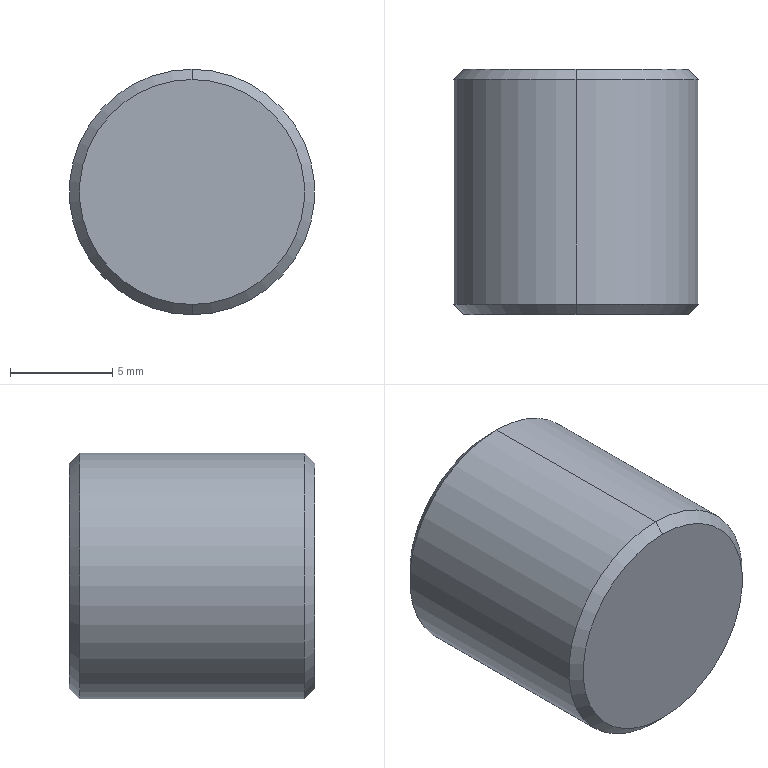Part | NX | features solid 2 | 1 solid | 20 faces | box 12 x 12 x 12 mm | volume 1208 mm3 | plane 14 | cone 4 | cylinder 2 | commonest cylinder face diameters 12 x2
STEP:
#1=CARTESIAN_POINT('',(240.5,-206.,53.));
#2=VERTEX_POINT('',#1);
#3=CARTESIAN_POINT('',(240.5,-206.,42.));
#4=VERTEX_POINT('',#3);
#5=CARTESIAN_POINT('',(240.5,-206.,47.5));
#6=DIRECTION('',(0.,1.,0.));
#7=DIRECTION('',(0.,0.,1.));
#8=AXIS2_PLACEMENT_3D('',#5,#6,#7);
#9=CIRCLE('',#8,5.5);
#10=EDGE_CURVE('',#2,#4,#9,.T.);
#11=ORIENTED_EDGE('',*,*,#10,.F.);
#12=CARTESIAN_POINT('',(240.5,-206.,47.5));
#13=DIRECTION('',(0.,-1.,0.));
#14=DIRECTION('',(0.,0.,1.));
#15=AXIS2_PLACEMENT_3D('',#12,#13,#14);
#16=CIRCLE('',#15,5.5);
#17=EDGE_CURVE('',#2,#4,#16,.T.);
#18=ORIENTED_EDGE('',*,*,#17,.T.);
#19=EDGE_LOOP('',(#11,#18));
#20=FACE_BOUND('',#19,.T.);
#21=CARTESIAN_POINT('',(240.5,-206.,47.5));
#22=DIRECTION('',(0.,1.,0.));
#23=DIRECTION('',(0.,0.,-1.));
#24=AXIS2_PLACEMENT_3D('',#21,#22,#23);
#25=PLANE('',#24);
#26=ADVANCED_FACE('',(#20),#25,.F.);
#27=CARTESIAN_POINT('',(240.5,-205.5,53.5));
#28=VERTEX_POINT('',#27);
#29=CARTESIAN_POINT('',(240.5,-206.,53.));
#30=DIRECTION('',(0.,0.7071,0.7071));
#31=VECTOR('',#30,1000.);
#32=LINE('',#29,#31);
#33=EDGE_CURVE('',#28,#2,#32,.F.);
#34=ORIENTED_EDGE('',*,*,#33,.F.);
#35=CARTESIAN_POINT('',(240.5,-205.5,41.5));
#36=VERTEX_POINT('',#35);
#37=CARTESIAN_POINT('',(240.5,-205.5,47.5));
#38=DIRECTION('',(0.,-1.,0.));
#39=DIRECTION('',(0.,0.,1.));
#40=AXIS2_PLACEMENT_3D('',#37,#38,#39);
#41=CIRCLE('',#40,6.);
#42=EDGE_CURVE('',#28,#36,#41,.T.);
#43=ORIENTED_EDGE('',*,*,#42,.T.);
#44=CARTESIAN_POINT('',(240.5,-206.,42.));
#45=DIRECTION('',(0.,0.7071,-0.7071));
#46=VECTOR('',#45,1000.);
#47=LINE('',#44,#46);
#48=EDGE_CURVE('',#4,#36,#47,.T.);
#49=ORIENTED_EDGE('',*,*,#48,.F.);
#50=ORIENTED_EDGE('',*,*,#17,.F.);
#51=EDGE_LOOP('',(#34,#43,#49,#50));
#52=FACE_BOUND('',#51,.T.);
#53=CARTESIAN_POINT('',(240.5,-205.75,47.5));
#54=DIRECTION('',(0.,1.,0.));
#55=DIRECTION('',(0.,0.,-1.));
#56=AXIS2_PLACEMENT_3D('',#53,#54,#55);
#57=CONICAL_SURFACE('',#56,5.75,0.7854);
#58=ADVANCED_FACE('',(#52),#57,.T.);
#59=ORIENTED_EDGE('',*,*,#48,.T.);
#60=CARTESIAN_POINT('',(240.5,-205.5,47.5));
#61=DIRECTION('',(0.,1.,0.));
#62=DIRECTION('',(0.,0.,1.));
#63=AXIS2_PLACEMENT_3D('',#60,#61,#62);
#64=CIRCLE('',#63,6.);
#65=EDGE_CURVE('',#28,#36,#64,.T.);
#66=ORIENTED_EDGE('',*,*,#65,.F.);
#67=ORIENTED_EDGE('',*,*,#33,.T.);
#68=ORIENTED_EDGE('',*,*,#10,.T.);
#69=EDGE_LOOP('',(#59,#66,#67,#68));
#70=FACE_BOUND('',#69,.T.);
#71=CARTESIAN_POINT('',(240.5,-205.75,47.5));
#72=DIRECTION('',(0.,1.,0.));
#73=DIRECTION('',(0.,0.,-1.));
#74=AXIS2_PLACEMENT_3D('',#71,#72,#73);
#75=CONICAL_SURFACE('',#74,5.75,0.7854);
#76=ADVANCED_FACE('',(#70),#75,.T.);
#77=ORIENTED_EDGE('',*,*,#65,.T.);
#78=CARTESIAN_POINT('',(240.5,-194.5,41.5));
#79=VERTEX_POINT('',#78);
#80=CARTESIAN_POINT('',(240.5,-194.5,41.5));
#81=DIRECTION('',(0.,-1.,0.));
#82=VECTOR('',#81,1000.);
#83=LINE('',#80,#82);
#84=EDGE_CURVE('',#36,#79,#83,.F.);
#85=ORIENTED_EDGE('',*,*,#84,.T.);
#86=CARTESIAN_POINT('',(240.5,-194.5,53.5));
#87=VERTEX_POINT('',#86);
#88=CARTESIAN_POINT('',(240.5,-194.5,47.5));
#89=DIRECTION('',(0.,1.,0.));
#90=DIRECTION('',(0.,0.,1.));
#91=AXIS2_PLACEMENT_3D('',#88,#89,#90);
#92=CIRCLE('',#91,6.);
#93=EDGE_CURVE('',#87,#79,#92,.T.);
#94=ORIENTED_EDGE('',*,*,#93,.F.);
#95=CARTESIAN_POINT('',(240.5,-194.5,53.5));
#96=DIRECTION('',(0.,-1.,0.));
#97=VECTOR('',#96,1000.);
#98=LINE('',#95,#97);
#99=EDGE_CURVE('',#87,#28,#98,.T.);
#100=ORIENTED_EDGE('',*,*,#99,.T.);
#101=EDGE_LOOP('',(#77,#85,#94,#100));
#102=FACE_BOUND('',#101,.T.);
#103=CARTESIAN_POINT('',(240.5,-206.6,47.5));
#104=DIRECTION('',(0.,1.,0.));
#105=DIRECTION('',(0.,0.,-1.));
#106=AXIS2_PLACEMENT_3D('',#103,#104,#105);
#107=CYLINDRICAL_SURFACE('',#106,6.);
#108=ADVANCED_FACE('',(#102),#107,.T.);
#109=CARTESIAN_POINT('',(240.5,-194.5,47.5));
#110=DIRECTION('',(0.,-1.,0.));
#111=DIRECTION('',(0.,0.,1.));
#112=AXIS2_PLACEMENT_3D('',#109,#110,#111);
#113=CIRCLE('',#112,6.);
#114=EDGE_CURVE('',#87,#79,#113,.T.);
#115=ORIENTED_EDGE('',*,*,#114,.T.);
#116=ORIENTED_EDGE('',*,*,#84,.F.);
#117=ORIENTED_EDGE('',*,*,#42,.F.);
#118=ORIENTED_EDGE('',*,*,#99,.F.);
#119=EDGE_LOOP('',(#115,#116,#117,#118));
#120=FACE_BOUND('',#119,.T.);
#121=CARTESIAN_POINT('',(240.5,-206.6,47.5));
#122=DIRECTION('',(0.,1.,0.));
#123=DIRECTION('',(0.,0.,-1.));
#124=AXIS2_PLACEMENT_3D('',#121,#122,#123);
#125=CYLINDRICAL_SURFACE('',#124,6.);
#126=ADVANCED_FACE('',(#120),#125,.T.);
#127=CARTESIAN_POINT('',(240.5,-194.,53.));
#128=VERTEX_POINT('',#127);
#129=CARTESIAN_POINT('',(240.5,-194.5,53.5));
#130=DIRECTION('',(0.,0.7071,-0.7071));
#131=VECTOR('',#130,1000.);
#132=LINE('',#129,#131);
#133=EDGE_CURVE('',#87,#128,#132,.T.);
#134=ORIENTED_EDGE('',*,*,#133,.T.);
#135=CARTESIAN_POINT('',(240.5,-194.,42.));
#136=VERTEX_POINT('',#135);
#137=CARTESIAN_POINT('',(240.5,-194.,47.5));
#138=DIRECTION('',(0.,-1.,0.));
#139=DIRECTION('',(0.,0.,1.));
#140=AXIS2_PLACEMENT_3D('',#137,#138,#139);
#141=CIRCLE('',#140,5.5);
#142=EDGE_CURVE('',#128,#136,#141,.T.);
#143=ORIENTED_EDGE('',*,*,#142,.T.);
#144=CARTESIAN_POINT('',(240.5,-194.5,41.5));
#145=DIRECTION('',(0.,0.7071,0.7071));
#146=VECTOR('',#145,1000.);
#147=LINE('',#144,#146);
#148=EDGE_CURVE('',#136,#79,#147,.F.);
#149=ORIENTED_EDGE('',*,*,#148,.T.);
#150=ORIENTED_EDGE('',*,*,#114,.F.);
#151=EDGE_LOOP('',(#134,#143,#149,#150));
#152=FACE_BOUND('',#151,.T.);
#153=CARTESIAN_POINT('',(240.5,-194.25,47.5));
#154=DIRECTION('',(0.,-1.,0.));
#155=DIRECTION('',(0.,0.,1.));
#156=AXIS2_PLACEMENT_3D('',#153,#154,#155);
#157=CONICAL_SURFACE('',#156,5.75,0.7854);
#158=ADVANCED_FACE('',(#152),#157,.T.);
#159=ORIENTED_EDGE('',*,*,#148,.F.);
#160=CARTESIAN_POINT('',(240.5,-194.,47.5));
#161=DIRECTION('',(0.,1.,0.));
#162=DIRECTION('',(0.,0.,1.));
#163=AXIS2_PLACEMENT_3D('',#160,#161,#162);
#164=CIRCLE('',#163,5.5);
#165=EDGE_CURVE('',#128,#136,#164,.T.);
#166=ORIENTED_EDGE('',*,*,#165,.F.);
#167=ORIENTED_EDGE('',*,*,#133,.F.);
#168=ORIENTED_EDGE('',*,*,#93,.T.);
#169=EDGE_LOOP('',(#159,#166,#167,#168));
#170=FACE_BOUND('',#169,.T.);
#171=CARTESIAN_POINT('',(240.5,-194.25,47.5));
#172=DIRECTION('',(0.,-1.,0.));
#173=DIRECTION('',(0.,0.,1.));
#174=AXIS2_PLACEMENT_3D('',#171,#172,#173);
#175=CONICAL_SURFACE('',#174,5.75,0.7854);
#176=ADVANCED_FACE('',(#170),#175,.T.);
#177=ORIENTED_EDGE('',*,*,#165,.T.);
#178=ORIENTED_EDGE('',*,*,#142,.F.);
#179=EDGE_LOOP('',(#177,#178));
#180=FACE_BOUND('',#179,.T.);
#181=CARTESIAN_POINT('',(240.5,-194.,44.036));
#182=VERTEX_POINT('',#181);
#183=CARTESIAN_POINT('',(237.5,-194.,45.768));
#184=VERTEX_POINT('',#183);
#185=CARTESIAN_POINT('',(240.5,-194.,44.036));
#186=DIRECTION('',(-0.866,0.,0.5));
#187=VECTOR('',#186,1000.);
#188=LINE('',#185,#187);
#189=EDGE_CURVE('',#182,#184,#188,.T.);
#190=ORIENTED_EDGE('',*,*,#189,.F.);
#191=CARTESIAN_POINT('',(243.5,-194.,45.768));
#192=VERTEX_POINT('',#191);
#193=CARTESIAN_POINT('',(243.5,-194.,45.768));
#194=DIRECTION('',(-0.866,0.,-0.5));
#195=VECTOR('',#194,1000.);
#196=LINE('',#193,#195);
#197=EDGE_CURVE('',#192,#182,#196,.T.);
#198=ORIENTED_EDGE('',*,*,#197,.F.);
#199=CARTESIAN_POINT('',(243.5,-194.,49.232));
#200=VERTEX_POINT('',#199);
#201=CARTESIAN_POINT('',(243.5,-194.,49.232));
#202=DIRECTION('',(0.,0.,-1.));
#203=VECTOR('',#202,1000.);
#204=LINE('',#201,#203);
#205=EDGE_CURVE('',#200,#192,#204,.T.);
#206=ORIENTED_EDGE('',*,*,#205,.F.);
#207=CARTESIAN_POINT('',(240.5,-194.,50.964));
#208=VERTEX_POINT('',#207);
#209=CARTESIAN_POINT('',(240.5,-194.,50.964));
#210=DIRECTION('',(0.866,0.,-0.5));
#211=VECTOR('',#210,1000.);
#212=LINE('',#209,#211);
#213=EDGE_CURVE('',#208,#200,#212,.T.);
#214=ORIENTED_EDGE('',*,*,#213,.F.);
#215=CARTESIAN_POINT('',(237.5,-194.,49.232));
#216=VERTEX_POINT('',#215);
#217=CARTESIAN_POINT('',(237.5,-194.,49.232));
#218=DIRECTION('',(0.866,0.,0.5));
#219=VECTOR('',#218,1000.);
#220=LINE('',#217,#219);
#221=EDGE_CURVE('',#216,#208,#220,.T.);
#222=ORIENTED_EDGE('',*,*,#221,.F.);
#223=CARTESIAN_POINT('',(237.5,-194.,45.768));
#224=DIRECTION('',(0.,0.,1.));
#225=VECTOR('',#224,1000.);
#226=LINE('',#223,#225);
#227=EDGE_CURVE('',#184,#216,#226,.T.);
#228=ORIENTED_EDGE('',*,*,#227,.F.);
#229=EDGE_LOOP('',(#190,#198,#206,#214,#222,#228));
#230=FACE_BOUND('',#229,.T.);
#231=CARTESIAN_POINT('',(240.5,-194.,47.5));
#232=DIRECTION('',(0.,1.,0.));
#233=DIRECTION('',(0.,0.,-1.));
#234=AXIS2_PLACEMENT_3D('',#231,#232,#233);
#235=PLANE('',#234);
#236=ADVANCED_FACE('',(#180,#230),#235,.T.);
#237=CARTESIAN_POINT('',(237.5,-198.,45.768));
#238=VERTEX_POINT('',#237);
#239=CARTESIAN_POINT('',(237.5,-194.,45.768));
#240=DIRECTION('',(0.,-1.,0.));
#241=VECTOR('',#240,1000.);
#242=LINE('',#239,#241);
#243=EDGE_CURVE('',#184,#238,#242,.T.);
#244=ORIENTED_EDGE('',*,*,#243,.F.);
#245=ORIENTED_EDGE('',*,*,#227,.T.);
#246=CARTESIAN_POINT('',(237.5,-198.,49.232));
#247=VERTEX_POINT('',#246);
#248=CARTESIAN_POINT('',(237.5,-194.,49.232));
#249=DIRECTION('',(0.,-1.,0.));
#250=VECTOR('',#249,1000.);
#251=LINE('',#248,#250);
#252=EDGE_CURVE('',#216,#247,#251,.T.);
#253=ORIENTED_EDGE('',*,*,#252,.T.);
#254=CARTESIAN_POINT('',(237.5,-198.,45.768));
#255=DIRECTION('',(0.,0.,1.));
#256=VECTOR('',#255,1000.);
#257=LINE('',#254,#256);
#258=EDGE_CURVE('',#238,#247,#257,.T.);
#259=ORIENTED_EDGE('',*,*,#258,.F.);
#260=EDGE_LOOP('',(#244,#245,#253,#259));
#261=FACE_BOUND('',#260,.T.);
#262=CARTESIAN_POINT('',(237.5,-194.,45.768));
#263=DIRECTION('',(-1.,0.,0.));
#264=DIRECTION('',(0.,0.,1.));
#265=AXIS2_PLACEMENT_3D('',#262,#263,#264);
#266=PLANE('',#265);
#267=ADVANCED_FACE('',(#261),#266,.F.);
#268=CARTESIAN_POINT('',(240.5,-199.5,47.5));
#269=VERTEX_POINT('',#268);
#270=CARTESIAN_POINT('',(240.5,-199.5,47.5));
#271=DIRECTION('',(-0.7947,0.3974,0.4588));
#272=VECTOR('',#271,1000.);
#273=LINE('',#270,#272);
#274=EDGE_CURVE('',#269,#247,#273,.T.);
#275=ORIENTED_EDGE('',*,*,#274,.F.);
#276=CARTESIAN_POINT('',(240.5,-199.5,47.5));
#277=DIRECTION('',(-0.7947,0.3974,-0.4588));
#278=VECTOR('',#277,1000.);
#279=LINE('',#276,#278);
#280=EDGE_CURVE('',#269,#238,#279,.T.);
#281=ORIENTED_EDGE('',*,*,#280,.T.);
#282=ORIENTED_EDGE('',*,*,#258,.T.);
#283=EDGE_LOOP('',(#275,#281,#282));
#284=FACE_BOUND('',#283,.T.);
#285=CARTESIAN_POINT('',(239.,-198.75,47.5));
#286=DIRECTION('',(-0.4472,-0.8944,0.));
#287=DIRECTION('',(-0.8944,0.4472,0.));
#288=AXIS2_PLACEMENT_3D('',#285,#286,#287);
#289=PLANE('',#288);
#290=ADVANCED_FACE('',(#284),#289,.F.);
#291=ORIENTED_EDGE('',*,*,#280,.F.);
#292=CARTESIAN_POINT('',(240.5,-198.,44.036));
#293=VERTEX_POINT('',#292);
#294=CARTESIAN_POINT('',(240.5,-199.5,47.5));
#295=DIRECTION('',(0.,0.3974,-0.9177));
#296=VECTOR('',#295,1000.);
#297=LINE('',#294,#296);
#298=EDGE_CURVE('',#269,#293,#297,.T.);
#299=ORIENTED_EDGE('',*,*,#298,.T.);
#300=CARTESIAN_POINT('',(240.5,-198.,44.036));
#301=DIRECTION('',(-0.866,0.,0.5));
#302=VECTOR('',#301,1000.);
#303=LINE('',#300,#302);
#304=EDGE_CURVE('',#293,#238,#303,.T.);
#305=ORIENTED_EDGE('',*,*,#304,.T.);
#306=EDGE_LOOP('',(#291,#299,#305));
#307=FACE_BOUND('',#306,.T.);
#308=CARTESIAN_POINT('',(239.75,-198.75,46.201));
#309=DIRECTION('',(-0.2236,-0.8944,-0.3873));
#310=DIRECTION('',(0.,-0.3974,0.9177));
#311=AXIS2_PLACEMENT_3D('',#308,#309,#310);
#312=PLANE('',#311);
#313=ADVANCED_FACE('',(#307),#312,.F.);
#314=CARTESIAN_POINT('',(240.5,-194.,44.036));
#315=DIRECTION('',(0.,-1.,0.));
#316=VECTOR('',#315,1000.);
#317=LINE('',#314,#316);
#318=EDGE_CURVE('',#182,#293,#317,.T.);
#319=ORIENTED_EDGE('',*,*,#318,.F.);
#320=ORIENTED_EDGE('',*,*,#189,.T.);
#321=ORIENTED_EDGE('',*,*,#243,.T.);
#322=ORIENTED_EDGE('',*,*,#304,.F.);
#323=EDGE_LOOP('',(#319,#320,#321,#322));
#324=FACE_BOUND('',#323,.T.);
#325=CARTESIAN_POINT('',(240.5,-194.,44.036));
#326=DIRECTION('',(-0.5,0.,-0.866));
#327=DIRECTION('',(-0.866,0.,0.5));
#328=AXIS2_PLACEMENT_3D('',#325,#326,#327);
#329=PLANE('',#328);
#330=ADVANCED_FACE('',(#324),#329,.F.);
#331=CARTESIAN_POINT('',(243.5,-198.,45.768));
#332=VERTEX_POINT('',#331);
#333=CARTESIAN_POINT('',(243.5,-194.,45.768));
#334=DIRECTION('',(0.,-1.,0.));
#335=VECTOR('',#334,1000.);
#336=LINE('',#333,#335);
#337=EDGE_CURVE('',#192,#332,#336,.T.);
#338=ORIENTED_EDGE('',*,*,#337,.F.);
#339=ORIENTED_EDGE('',*,*,#197,.T.);
#340=ORIENTED_EDGE('',*,*,#318,.T.);
#341=CARTESIAN_POINT('',(243.5,-198.,45.768));
#342=DIRECTION('',(-0.866,0.,-0.5));
#343=VECTOR('',#342,1000.);
#344=LINE('',#341,#343);
#345=EDGE_CURVE('',#332,#293,#344,.T.);
#346=ORIENTED_EDGE('',*,*,#345,.F.);
#347=EDGE_LOOP('',(#338,#339,#340,#346));
#348=FACE_BOUND('',#347,.T.);
#349=CARTESIAN_POINT('',(243.5,-194.,45.768));
#350=DIRECTION('',(0.5,0.,-0.866));
#351=DIRECTION('',(-0.866,0.,-0.5));
#352=AXIS2_PLACEMENT_3D('',#349,#350,#351);
#353=PLANE('',#352);
#354=ADVANCED_FACE('',(#348),#353,.F.);
#355=ORIENTED_EDGE('',*,*,#298,.F.);
#356=CARTESIAN_POINT('',(240.5,-199.5,47.5));
#357=DIRECTION('',(0.7947,0.3974,-0.4588));
#358=VECTOR('',#357,1000.);
#359=LINE('',#356,#358);
#360=EDGE_CURVE('',#269,#332,#359,.T.);
#361=ORIENTED_EDGE('',*,*,#360,.T.);
#362=ORIENTED_EDGE('',*,*,#345,.T.);
#363=EDGE_LOOP('',(#355,#361,#362));
#364=FACE_BOUND('',#363,.T.);
#365=CARTESIAN_POINT('',(241.25,-198.75,46.201));
#366=DIRECTION('',(0.2236,-0.8944,-0.3873));
#367=DIRECTION('',(0.,-0.3974,0.9177));
#368=AXIS2_PLACEMENT_3D('',#365,#366,#367);
#369=PLANE('',#368);
#370=ADVANCED_FACE('',(#364),#369,.F.);
#371=ORIENTED_EDGE('',*,*,#360,.F.);
#372=CARTESIAN_POINT('',(243.5,-198.,49.232));
#373=VERTEX_POINT('',#372);
#374=CARTESIAN_POINT('',(240.5,-199.5,47.5));
#375=DIRECTION('',(0.7947,0.3974,0.4588));
#376=VECTOR('',#375,1000.);
#377=LINE('',#374,#376);
#378=EDGE_CURVE('',#269,#373,#377,.T.);
#379=ORIENTED_EDGE('',*,*,#378,.T.);
#380=CARTESIAN_POINT('',(243.5,-198.,49.232));
#381=DIRECTION('',(0.,0.,-1.));
#382=VECTOR('',#381,1000.);
#383=LINE('',#380,#382);
#384=EDGE_CURVE('',#373,#332,#383,.T.);
#385=ORIENTED_EDGE('',*,*,#384,.T.);
#386=EDGE_LOOP('',(#371,#379,#385));
#387=FACE_BOUND('',#386,.T.);
#388=CARTESIAN_POINT('',(242.,-198.75,47.5));
#389=DIRECTION('',(0.4472,-0.8944,0.));
#390=DIRECTION('',(-0.8944,-0.4472,0.));
#391=AXIS2_PLACEMENT_3D('',#388,#389,#390);
#392=PLANE('',#391);
#393=ADVANCED_FACE('',(#387),#392,.F.);
#394=CARTESIAN_POINT('',(243.5,-194.,49.232));
#395=DIRECTION('',(0.,-1.,0.));
#396=VECTOR('',#395,1000.);
#397=LINE('',#394,#396);
#398=EDGE_CURVE('',#200,#373,#397,.T.);
#399=ORIENTED_EDGE('',*,*,#398,.F.);
#400=ORIENTED_EDGE('',*,*,#205,.T.);
#401=ORIENTED_EDGE('',*,*,#337,.T.);
#402=ORIENTED_EDGE('',*,*,#384,.F.);
#403=EDGE_LOOP('',(#399,#400,#401,#402));
#404=FACE_BOUND('',#403,.T.);
#405=CARTESIAN_POINT('',(243.5,-194.,49.232));
#406=DIRECTION('',(1.,0.,0.));
#407=DIRECTION('',(0.,0.,-1.));
#408=AXIS2_PLACEMENT_3D('',#405,#406,#407);
#409=PLANE('',#408);
#410=ADVANCED_FACE('',(#404),#409,.F.);
#411=CARTESIAN_POINT('',(240.5,-198.,50.964));
#412=VERTEX_POINT('',#411);
#413=CARTESIAN_POINT('',(240.5,-194.,50.964));
#414=DIRECTION('',(0.,-1.,0.));
#415=VECTOR('',#414,1000.);
#416=LINE('',#413,#415);
#417=EDGE_CURVE('',#208,#412,#416,.T.);
#418=ORIENTED_EDGE('',*,*,#417,.F.);
#419=ORIENTED_EDGE('',*,*,#213,.T.);
#420=ORIENTED_EDGE('',*,*,#398,.T.);
#421=CARTESIAN_POINT('',(240.5,-198.,50.964));
#422=DIRECTION('',(0.866,0.,-0.5));
#423=VECTOR('',#422,1000.);
#424=LINE('',#421,#423);
#425=EDGE_CURVE('',#412,#373,#424,.T.);
#426=ORIENTED_EDGE('',*,*,#425,.F.);
#427=EDGE_LOOP('',(#418,#419,#420,#426));
#428=FACE_BOUND('',#427,.T.);
#429=CARTESIAN_POINT('',(240.5,-194.,50.964));
#430=DIRECTION('',(0.5,0.,0.866));
#431=DIRECTION('',(0.866,0.,-0.5));
#432=AXIS2_PLACEMENT_3D('',#429,#430,#431);
#433=PLANE('',#432);
#434=ADVANCED_FACE('',(#428),#433,.F.);
#435=ORIENTED_EDGE('',*,*,#378,.F.);
#436=CARTESIAN_POINT('',(240.5,-199.5,47.5));
#437=DIRECTION('',(0.,0.3974,0.9177));
#438=VECTOR('',#437,1000.);
#439=LINE('',#436,#438);
#440=EDGE_CURVE('',#269,#412,#439,.T.);
#441=ORIENTED_EDGE('',*,*,#440,.T.);
#442=ORIENTED_EDGE('',*,*,#425,.T.);
#443=EDGE_LOOP('',(#435,#441,#442));
#444=FACE_BOUND('',#443,.T.);
#445=CARTESIAN_POINT('',(241.25,-198.75,48.799));
#446=DIRECTION('',(0.2236,-0.8944,0.3873));
#447=DIRECTION('',(0.,0.3974,0.9177));
#448=AXIS2_PLACEMENT_3D('',#445,#446,#447);
#449=PLANE('',#448);
#450=ADVANCED_FACE('',(#444),#449,.F.);
#451=ORIENTED_EDGE('',*,*,#440,.F.);
#452=ORIENTED_EDGE('',*,*,#274,.T.);
#453=CARTESIAN_POINT('',(237.5,-198.,49.232));
#454=DIRECTION('',(0.866,0.,0.5));
#455=VECTOR('',#454,1000.);
#456=LINE('',#453,#455);
#457=EDGE_CURVE('',#247,#412,#456,.T.);
#458=ORIENTED_EDGE('',*,*,#457,.T.);
#459=EDGE_LOOP('',(#451,#452,#458));
#460=FACE_BOUND('',#459,.T.);
#461=CARTESIAN_POINT('',(239.75,-198.75,48.799));
#462=DIRECTION('',(-0.2236,-0.8944,0.3873));
#463=DIRECTION('',(0.,0.3974,0.9177));
#464=AXIS2_PLACEMENT_3D('',#461,#462,#463);
#465=PLANE('',#464);
#466=ADVANCED_FACE('',(#460),#465,.F.);
#467=ORIENTED_EDGE('',*,*,#252,.F.);
#468=ORIENTED_EDGE('',*,*,#221,.T.);
#469=ORIENTED_EDGE('',*,*,#417,.T.);
#470=ORIENTED_EDGE('',*,*,#457,.F.);
#471=EDGE_LOOP('',(#467,#468,#469,#470));
#472=FACE_BOUND('',#471,.T.);
#473=CARTESIAN_POINT('',(237.5,-194.,49.232));
#474=DIRECTION('',(-0.5,0.,0.866));
#475=DIRECTION('',(0.866,0.,0.5));
#476=AXIS2_PLACEMENT_3D('',#473,#474,#475);
#477=PLANE('',#476);
#478=ADVANCED_FACE('',(#472),#477,.F.);
#479=CLOSED_SHELL('',(#26,#58,#76,#108,#126,#158,#176,#236,#267,#290,#313,#330,#354,#370,#393,#410,#434,#450,#466,#478));
#480=MANIFOLD_SOLID_BREP('',#479);
#481=(LENGTH_UNIT()NAMED_UNIT(*)SI_UNIT(.MILLI.,.METRE.));
#482=UNCERTAINTY_MEASURE_WITH_UNIT(LENGTH_MEASURE(0.00001),#481,'','');
#483=(NAMED_UNIT(*)PLANE_ANGLE_UNIT()SI_UNIT($,.RADIAN.));
#484=(NAMED_UNIT(*)SI_UNIT($,.STERADIAN.)SOLID_ANGLE_UNIT());
#485=(GEOMETRIC_REPRESENTATION_CONTEXT(3)GLOBAL_UNCERTAINTY_ASSIGNED_CONTEXT((#482))GLOBAL_UNIT_ASSIGNED_CONTEXT((#481,#483,#484))REPRESENTATION_CONTEXT('',''));
#486=ADVANCED_BREP_SHAPE_REPRESENTATION('',(#480),#485);